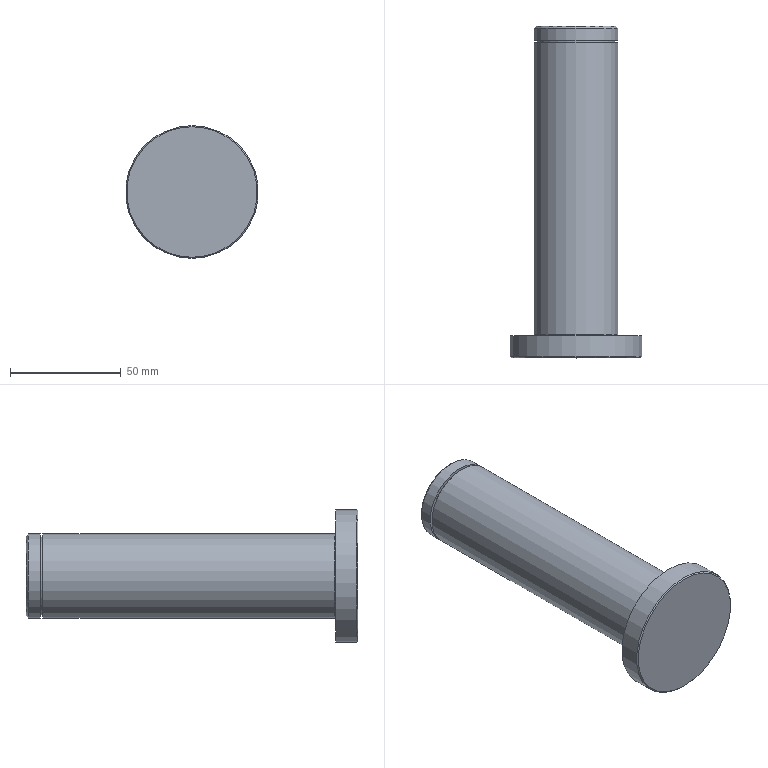Part | NX | features DATUM_CSYS 3, CHAMFER 2, SKETCH 2, SWP104 2, BLEND 1, Intersection Curve 1 | 1 solid | 12 faces | box 60 x 150 x 60 mm | volume 186798 mm3 | plane 5 | cylinder 4 | cone 2 | torus 1 | commonest cylinder face diameters 38 x2 35.2 x1 60 x1
STEP:
#1=CARTESIAN_POINT('',(0.,-10.,29.5));
#2=VERTEX_POINT('',#1);
#3=CARTESIAN_POINT('',(0.,-10.,0.));
#4=DIRECTION('',(0.,1.,0.));
#5=DIRECTION('',(0.,0.,1.));
#6=AXIS2_PLACEMENT_3D('',#3,#4,#5);
#7=CIRCLE('',#6,29.5);
#8=EDGE_CURVE('',#2,#2,#7,.F.);
#9=ORIENTED_EDGE('',*,*,#8,.T.);
#10=EDGE_LOOP('',(#9));
#11=FACE_BOUND('',#10,.T.);
#12=CARTESIAN_POINT('',(0.,-10.,0.));
#13=DIRECTION('',(0.,1.,0.));
#14=DIRECTION('',(0.,0.,1.));
#15=AXIS2_PLACEMENT_3D('',#12,#13,#14);
#16=PLANE('',#15);
#17=ADVANCED_FACE('',(#11),#16,.F.);
#18=CARTESIAN_POINT('',(0.,0.5,-19.));
#19=VERTEX_POINT('',#18);
#20=CARTESIAN_POINT('',(0.,0.5,0.));
#21=DIRECTION('',(0.,-1.,0.));
#22=DIRECTION('',(0.,0.,-1.));
#23=AXIS2_PLACEMENT_3D('',#20,#21,#22);
#24=CIRCLE('',#23,19.);
#25=EDGE_CURVE('',#19,#19,#24,.F.);
#26=ORIENTED_EDGE('',*,*,#25,.T.);
#27=EDGE_LOOP('',(#26));
#28=FACE_BOUND('',#27,.T.);
#29=CARTESIAN_POINT('',(0.,132.4,-19.));
#30=VERTEX_POINT('',#29);
#31=CARTESIAN_POINT('',(0.,132.4,0.));
#32=DIRECTION('',(0.,-1.,0.));
#33=DIRECTION('',(0.,0.,-1.));
#34=AXIS2_PLACEMENT_3D('',#31,#32,#33);
#35=CIRCLE('',#34,19.);
#36=EDGE_CURVE('',#30,#30,#35,.T.);
#37=ORIENTED_EDGE('',*,*,#36,.T.);
#38=EDGE_LOOP('',(#37));
#39=FACE_BOUND('',#38,.T.);
#40=CARTESIAN_POINT('',(0.,0.,0.));
#41=DIRECTION('',(0.,1.,0.));
#42=DIRECTION('',(0.,0.,1.));
#43=AXIS2_PLACEMENT_3D('',#40,#41,#42);
#44=CYLINDRICAL_SURFACE('',#43,19.);
#45=ADVANCED_FACE('',(#28,#39),#44,.T.);
#46=CARTESIAN_POINT('',(0.,0.,-19.5));
#47=VERTEX_POINT('',#46);
#48=CARTESIAN_POINT('',(0.,0.,0.));
#49=DIRECTION('',(0.,-1.,0.));
#50=DIRECTION('',(0.,0.,-1.));
#51=AXIS2_PLACEMENT_3D('',#48,#49,#50);
#52=CIRCLE('',#51,19.5);
#53=EDGE_CURVE('',#47,#47,#52,.T.);
#54=ORIENTED_EDGE('',*,*,#53,.T.);
#55=EDGE_LOOP('',(#54));
#56=FACE_BOUND('',#55,.T.);
#57=CARTESIAN_POINT('',(0.,0.,30.));
#58=VERTEX_POINT('',#57);
#59=CARTESIAN_POINT('',(0.,0.,0.));
#60=DIRECTION('',(0.,1.,0.));
#61=DIRECTION('',(0.,0.,1.));
#62=AXIS2_PLACEMENT_3D('',#59,#60,#61);
#63=CIRCLE('',#62,30.);
#64=EDGE_CURVE('',#58,#58,#63,.T.);
#65=ORIENTED_EDGE('',*,*,#64,.T.);
#66=EDGE_LOOP('',(#65));
#67=FACE_BOUND('',#66,.T.);
#68=CARTESIAN_POINT('',(0.,0.,30.));
#69=DIRECTION('',(0.,-1.,0.));
#70=DIRECTION('',(0.,0.,-1.));
#71=AXIS2_PLACEMENT_3D('',#68,#69,#70);
#72=PLANE('',#71);
#73=ADVANCED_FACE('',(#56,#67),#72,.F.);
#74=CARTESIAN_POINT('',(0.,-9.5,30.));
#75=VERTEX_POINT('',#74);
#76=CARTESIAN_POINT('',(0.,-9.5,0.));
#77=DIRECTION('',(0.,1.,0.));
#78=DIRECTION('',(0.,0.,1.));
#79=AXIS2_PLACEMENT_3D('',#76,#77,#78);
#80=CIRCLE('',#79,30.);
#81=EDGE_CURVE('',#75,#75,#80,.T.);
#82=ORIENTED_EDGE('',*,*,#81,.T.);
#83=EDGE_LOOP('',(#82));
#84=FACE_BOUND('',#83,.T.);
#85=ORIENTED_EDGE('',*,*,#64,.F.);
#86=EDGE_LOOP('',(#85));
#87=FACE_BOUND('',#86,.T.);
#88=CARTESIAN_POINT('',(0.,0.,0.));
#89=DIRECTION('',(0.,1.,0.));
#90=DIRECTION('',(0.,0.,1.));
#91=AXIS2_PLACEMENT_3D('',#88,#89,#90);
#92=CYLINDRICAL_SURFACE('',#91,30.);
#93=ADVANCED_FACE('',(#84,#87),#92,.T.);
#94=CARTESIAN_POINT('',(0.,132.4,-17.6));
#95=VERTEX_POINT('',#94);
#96=CARTESIAN_POINT('',(0.,132.4,0.));
#97=DIRECTION('',(0.,-1.,0.));
#98=DIRECTION('',(0.,0.,-1.));
#99=AXIS2_PLACEMENT_3D('',#96,#97,#98);
#100=CIRCLE('',#99,17.6);
#101=EDGE_CURVE('',#95,#95,#100,.F.);
#102=ORIENTED_EDGE('',*,*,#101,.F.);
#103=EDGE_LOOP('',(#102));
#104=FACE_BOUND('',#103,.T.);
#105=ORIENTED_EDGE('',*,*,#36,.F.);
#106=EDGE_LOOP('',(#105));
#107=FACE_BOUND('',#106,.T.);
#108=CARTESIAN_POINT('',(0.,132.4,19.));
#109=DIRECTION('',(0.,1.,0.));
#110=DIRECTION('',(0.,0.,1.));
#111=AXIS2_PLACEMENT_3D('',#108,#109,#110);
#112=PLANE('',#111);
#113=ADVANCED_FACE('',(#104,#107),#112,.T.);
#114=CARTESIAN_POINT('',(0.,133.5,-17.6));
#115=VERTEX_POINT('',#114);
#116=CARTESIAN_POINT('',(0.,133.5,0.));
#117=DIRECTION('',(0.,-1.,0.));
#118=DIRECTION('',(0.,0.,-1.));
#119=AXIS2_PLACEMENT_3D('',#116,#117,#118);
#120=CIRCLE('',#119,17.6);
#121=EDGE_CURVE('',#115,#115,#120,.F.);
#122=ORIENTED_EDGE('',*,*,#121,.F.);
#123=EDGE_LOOP('',(#122));
#124=FACE_BOUND('',#123,.T.);
#125=ORIENTED_EDGE('',*,*,#101,.T.);
#126=EDGE_LOOP('',(#125));
#127=FACE_BOUND('',#126,.T.);
#128=CARTESIAN_POINT('',(0.,0.,0.));
#129=DIRECTION('',(0.,-1.,0.));
#130=DIRECTION('',(0.,0.,-1.));
#131=AXIS2_PLACEMENT_3D('',#128,#129,#130);
#132=CYLINDRICAL_SURFACE('',#131,17.6);
#133=ADVANCED_FACE('',(#124,#127),#132,.T.);
#134=CARTESIAN_POINT('',(0.,133.5,-19.));
#135=VERTEX_POINT('',#134);
#136=CARTESIAN_POINT('',(0.,133.5,0.));
#137=DIRECTION('',(0.,-1.,0.));
#138=DIRECTION('',(0.,0.,-1.));
#139=AXIS2_PLACEMENT_3D('',#136,#137,#138);
#140=CIRCLE('',#139,19.);
#141=EDGE_CURVE('',#135,#135,#140,.T.);
#142=ORIENTED_EDGE('',*,*,#141,.T.);
#143=EDGE_LOOP('',(#142));
#144=FACE_BOUND('',#143,.T.);
#145=ORIENTED_EDGE('',*,*,#121,.T.);
#146=EDGE_LOOP('',(#145));
#147=FACE_BOUND('',#146,.T.);
#148=CARTESIAN_POINT('',(0.,133.5,17.6));
#149=DIRECTION('',(0.,-1.,0.));
#150=DIRECTION('',(0.,0.,-1.));
#151=AXIS2_PLACEMENT_3D('',#148,#149,#150);
#152=PLANE('',#151);
#153=ADVANCED_FACE('',(#144,#147),#152,.T.);
#154=CARTESIAN_POINT('',(0.,140.,18.));
#155=VERTEX_POINT('',#154);
#156=CARTESIAN_POINT('',(0.,140.,0.));
#157=DIRECTION('',(0.,1.,0.));
#158=DIRECTION('',(0.,0.,1.));
#159=AXIS2_PLACEMENT_3D('',#156,#157,#158);
#160=CIRCLE('',#159,18.);
#161=EDGE_CURVE('',#155,#155,#160,.T.);
#162=ORIENTED_EDGE('',*,*,#161,.T.);
#163=EDGE_LOOP('',(#162));
#164=FACE_BOUND('',#163,.T.);
#165=CARTESIAN_POINT('',(0.,140.,0.));
#166=DIRECTION('',(0.,1.,0.));
#167=DIRECTION('',(0.,0.,1.));
#168=AXIS2_PLACEMENT_3D('',#165,#166,#167);
#169=PLANE('',#168);
#170=ADVANCED_FACE('',(#164),#169,.T.);
#171=CARTESIAN_POINT('',(0.,139.,19.));
#172=VERTEX_POINT('',#171);
#173=CARTESIAN_POINT('',(0.,139.,0.));
#174=DIRECTION('',(0.,1.,0.));
#175=DIRECTION('',(0.,0.,1.));
#176=AXIS2_PLACEMENT_3D('',#173,#174,#175);
#177=CIRCLE('',#176,19.);
#178=EDGE_CURVE('',#172,#172,#177,.F.);
#179=ORIENTED_EDGE('',*,*,#178,.T.);
#180=EDGE_LOOP('',(#179));
#181=FACE_BOUND('',#180,.T.);
#182=ORIENTED_EDGE('',*,*,#141,.F.);
#183=EDGE_LOOP('',(#182));
#184=FACE_BOUND('',#183,.T.);
#185=CARTESIAN_POINT('',(0.,0.,0.));
#186=DIRECTION('',(0.,1.,0.));
#187=DIRECTION('',(0.,0.,1.));
#188=AXIS2_PLACEMENT_3D('',#185,#186,#187);
#189=CYLINDRICAL_SURFACE('',#188,19.);
#190=ADVANCED_FACE('',(#181,#184),#189,.T.);
#191=ORIENTED_EDGE('',*,*,#8,.F.);
#192=EDGE_LOOP('',(#191));
#193=FACE_BOUND('',#192,.T.);
#194=ORIENTED_EDGE('',*,*,#81,.F.);
#195=EDGE_LOOP('',(#194));
#196=FACE_BOUND('',#195,.T.);
#197=CARTESIAN_POINT('',(0.,-9.5,0.));
#198=DIRECTION('',(0.,1.,0.));
#199=DIRECTION('',(0.,0.,1.));
#200=AXIS2_PLACEMENT_3D('',#197,#198,#199);
#201=CONICAL_SURFACE('',#200,30.,0.7854);
#202=ADVANCED_FACE('',(#193,#196),#201,.T.);
#203=ORIENTED_EDGE('',*,*,#178,.F.);
#204=EDGE_LOOP('',(#203));
#205=FACE_BOUND('',#204,.T.);
#206=ORIENTED_EDGE('',*,*,#161,.F.);
#207=EDGE_LOOP('',(#206));
#208=FACE_BOUND('',#207,.T.);
#209=CARTESIAN_POINT('',(0.,140.,0.));
#210=DIRECTION('',(0.,-1.,0.));
#211=DIRECTION('',(0.,0.,-1.));
#212=AXIS2_PLACEMENT_3D('',#209,#210,#211);
#213=CONICAL_SURFACE('',#212,18.,0.7854);
#214=ADVANCED_FACE('',(#205,#208),#213,.T.);
#215=ORIENTED_EDGE('',*,*,#53,.F.);
#216=EDGE_LOOP('',(#215));
#217=FACE_BOUND('',#216,.T.);
#218=ORIENTED_EDGE('',*,*,#25,.F.);
#219=EDGE_LOOP('',(#218));
#220=FACE_BOUND('',#219,.T.);
#221=CARTESIAN_POINT('',(0.,0.5,0.));
#222=DIRECTION('',(0.,-1.,0.));
#223=DIRECTION('',(0.,0.,-1.));
#224=AXIS2_PLACEMENT_3D('',#221,#222,#223);
#225=TOROIDAL_SURFACE('',#224,19.5,0.5);
#226=ADVANCED_FACE('',(#217,#220),#225,.F.);
#227=CLOSED_SHELL('',(#17,#45,#73,#93,#113,#133,#153,#170,#190,#202,#214,#226));
#228=MANIFOLD_SOLID_BREP('',#227);
#229=(LENGTH_UNIT()NAMED_UNIT(*)SI_UNIT(.MILLI.,.METRE.));
#230=UNCERTAINTY_MEASURE_WITH_UNIT(LENGTH_MEASURE(0.00001),#229,'','');
#231=(NAMED_UNIT(*)PLANE_ANGLE_UNIT()SI_UNIT($,.RADIAN.));
#232=(NAMED_UNIT(*)SI_UNIT($,.STERADIAN.)SOLID_ANGLE_UNIT());
#233=(GEOMETRIC_REPRESENTATION_CONTEXT(3)GLOBAL_UNCERTAINTY_ASSIGNED_CONTEXT((#230))GLOBAL_UNIT_ASSIGNED_CONTEXT((#229,#231,#232))REPRESENTATION_CONTEXT('',''));
#234=ADVANCED_BREP_SHAPE_REPRESENTATION('',(#228),#233);